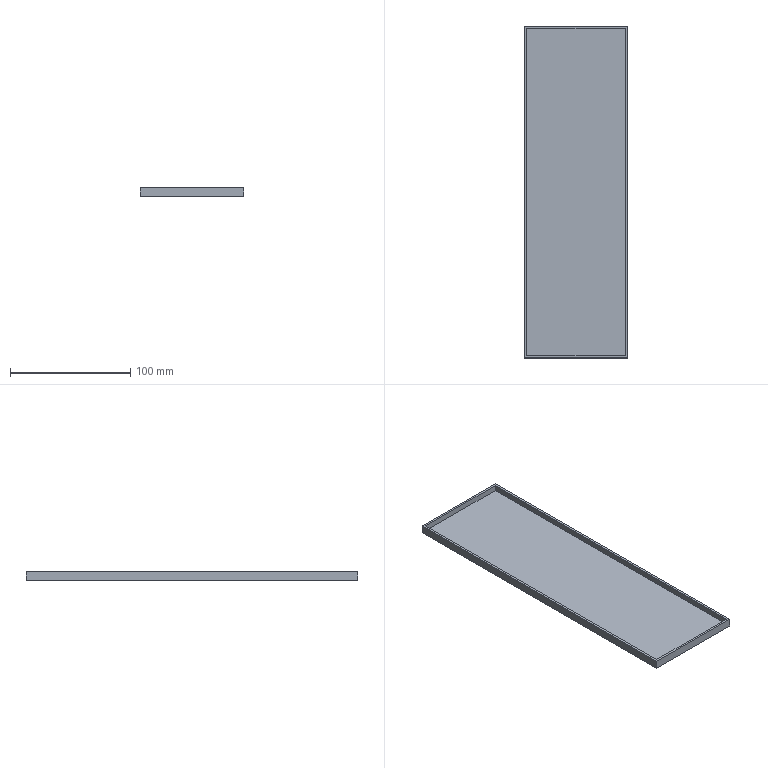Part | NX | features solid 2 | 1 solid | 11 faces | box 86 x 276 x 7 mm | volume 54632 mm3 | plane 11
STEP:
#1=CARTESIAN_POINT('',(348.,283.,-287.));
#2=VERTEX_POINT('',#1);
#3=CARTESIAN_POINT('',(348.,7.,-287.));
#4=VERTEX_POINT('',#3);
#5=CARTESIAN_POINT('',(348.,10.,-287.));
#6=DIRECTION('',(0.,-1.,0.));
#7=VECTOR('',#6,1000.);
#8=LINE('',#5,#7);
#9=EDGE_CURVE('',#2,#4,#8,.T.);
#10=ORIENTED_EDGE('',*,*,#9,.F.);
#11=CARTESIAN_POINT('',(348.,283.,-280.));
#12=VERTEX_POINT('',#11);
#13=CARTESIAN_POINT('',(348.,283.,-280.));
#14=DIRECTION('',(0.,0.,-1.));
#15=VECTOR('',#14,1000.);
#16=LINE('',#13,#15);
#17=EDGE_CURVE('',#12,#2,#16,.T.);
#18=ORIENTED_EDGE('',*,*,#17,.F.);
#19=CARTESIAN_POINT('',(348.,7.,-280.));
#20=VERTEX_POINT('',#19);
#21=CARTESIAN_POINT('',(348.,10.,-280.));
#22=DIRECTION('',(0.,-1.,0.));
#23=VECTOR('',#22,1000.);
#24=LINE('',#21,#23);
#25=EDGE_CURVE('',#12,#20,#24,.T.);
#26=ORIENTED_EDGE('',*,*,#25,.T.);
#27=CARTESIAN_POINT('',(348.,7.,-280.));
#28=DIRECTION('',(0.,0.,-1.));
#29=VECTOR('',#28,1000.);
#30=LINE('',#27,#29);
#31=EDGE_CURVE('',#20,#4,#30,.T.);
#32=ORIENTED_EDGE('',*,*,#31,.T.);
#33=EDGE_LOOP('',(#10,#18,#26,#32));
#34=FACE_BOUND('',#33,.T.);
#35=CARTESIAN_POINT('',(348.,290.,-280.));
#36=DIRECTION('',(1.,0.,0.));
#37=DIRECTION('',(0.,0.,-1.));
#38=AXIS2_PLACEMENT_3D('',#35,#36,#37);
#39=PLANE('',#38);
#40=ADVANCED_FACE('',(#34),#39,.T.);
#41=CARTESIAN_POINT('',(262.,7.,-287.));
#42=VERTEX_POINT('',#41);
#43=CARTESIAN_POINT('',(345.,7.,-287.));
#44=DIRECTION('',(-1.,0.,0.));
#45=VECTOR('',#44,1000.);
#46=LINE('',#43,#45);
#47=EDGE_CURVE('',#4,#42,#46,.T.);
#48=ORIENTED_EDGE('',*,*,#47,.F.);
#49=ORIENTED_EDGE('',*,*,#31,.F.);
#50=CARTESIAN_POINT('',(262.,7.,-280.));
#51=VERTEX_POINT('',#50);
#52=CARTESIAN_POINT('',(345.,7.,-280.));
#53=DIRECTION('',(-1.,0.,0.));
#54=VECTOR('',#53,1000.);
#55=LINE('',#52,#54);
#56=EDGE_CURVE('',#20,#51,#55,.T.);
#57=ORIENTED_EDGE('',*,*,#56,.T.);
#58=CARTESIAN_POINT('',(262.,7.,-280.));
#59=DIRECTION('',(0.,0.,-1.));
#60=VECTOR('',#59,1000.);
#61=LINE('',#58,#60);
#62=EDGE_CURVE('',#51,#42,#61,.T.);
#63=ORIENTED_EDGE('',*,*,#62,.T.);
#64=EDGE_LOOP('',(#48,#49,#57,#63));
#65=FACE_BOUND('',#64,.T.);
#66=CARTESIAN_POINT('',(345.,7.,-280.));
#67=DIRECTION('',(0.,-1.,0.));
#68=DIRECTION('',(0.,0.,-1.));
#69=AXIS2_PLACEMENT_3D('',#66,#67,#68);
#70=PLANE('',#69);
#71=ADVANCED_FACE('',(#65),#70,.T.);
#72=CARTESIAN_POINT('',(262.,283.,-287.));
#73=VERTEX_POINT('',#72);
#74=CARTESIAN_POINT('',(262.,10.,-287.));
#75=DIRECTION('',(0.,1.,0.));
#76=VECTOR('',#75,1000.);
#77=LINE('',#74,#76);
#78=EDGE_CURVE('',#42,#73,#77,.T.);
#79=ORIENTED_EDGE('',*,*,#78,.F.);
#80=ORIENTED_EDGE('',*,*,#62,.F.);
#81=CARTESIAN_POINT('',(262.,283.,-280.));
#82=VERTEX_POINT('',#81);
#83=CARTESIAN_POINT('',(262.,10.,-280.));
#84=DIRECTION('',(0.,1.,0.));
#85=VECTOR('',#84,1000.);
#86=LINE('',#83,#85);
#87=EDGE_CURVE('',#51,#82,#86,.T.);
#88=ORIENTED_EDGE('',*,*,#87,.T.);
#89=CARTESIAN_POINT('',(262.,283.,-280.));
#90=DIRECTION('',(0.,0.,-1.));
#91=VECTOR('',#90,1000.);
#92=LINE('',#89,#91);
#93=EDGE_CURVE('',#82,#73,#92,.T.);
#94=ORIENTED_EDGE('',*,*,#93,.T.);
#95=EDGE_LOOP('',(#79,#80,#88,#94));
#96=FACE_BOUND('',#95,.T.);
#97=CARTESIAN_POINT('',(262.,10.,-280.));
#98=DIRECTION('',(-1.,0.,0.));
#99=DIRECTION('',(0.,0.,1.));
#100=AXIS2_PLACEMENT_3D('',#97,#98,#99);
#101=PLANE('',#100);
#102=ADVANCED_FACE('',(#96),#101,.T.);
#103=CARTESIAN_POINT('',(345.,283.,-287.));
#104=DIRECTION('',(1.,0.,0.));
#105=VECTOR('',#104,1000.);
#106=LINE('',#103,#105);
#107=EDGE_CURVE('',#73,#2,#106,.T.);
#108=ORIENTED_EDGE('',*,*,#107,.F.);
#109=ORIENTED_EDGE('',*,*,#93,.F.);
#110=CARTESIAN_POINT('',(345.,283.,-280.));
#111=DIRECTION('',(1.,0.,0.));
#112=VECTOR('',#111,1000.);
#113=LINE('',#110,#112);
#114=EDGE_CURVE('',#82,#12,#113,.T.);
#115=ORIENTED_EDGE('',*,*,#114,.T.);
#116=ORIENTED_EDGE('',*,*,#17,.T.);
#117=EDGE_LOOP('',(#108,#109,#115,#116));
#118=FACE_BOUND('',#117,.T.);
#119=CARTESIAN_POINT('',(-690.,283.,-280.));
#120=DIRECTION('',(0.,1.,0.));
#121=DIRECTION('',(-1.,0.,0.));
#122=AXIS2_PLACEMENT_3D('',#119,#120,#121);
#123=PLANE('',#122);
#124=ADVANCED_FACE('',(#118),#123,.T.);
#125=CARTESIAN_POINT('',(264.,281.,-280.));
#126=VERTEX_POINT('',#125);
#127=CARTESIAN_POINT('',(346.,281.,-280.));
#128=VERTEX_POINT('',#127);
#129=CARTESIAN_POINT('',(345.,281.,-280.));
#130=DIRECTION('',(1.,0.,0.));
#131=VECTOR('',#130,1000.);
#132=LINE('',#129,#131);
#133=EDGE_CURVE('',#126,#128,#132,.T.);
#134=ORIENTED_EDGE('',*,*,#133,.T.);
#135=CARTESIAN_POINT('',(346.,9.,-280.));
#136=VERTEX_POINT('',#135);
#137=CARTESIAN_POINT('',(346.,10.,-280.));
#138=DIRECTION('',(0.,-1.,0.));
#139=VECTOR('',#138,1000.);
#140=LINE('',#137,#139);
#141=EDGE_CURVE('',#128,#136,#140,.T.);
#142=ORIENTED_EDGE('',*,*,#141,.T.);
#143=CARTESIAN_POINT('',(264.,9.,-280.));
#144=VERTEX_POINT('',#143);
#145=CARTESIAN_POINT('',(345.,9.,-280.));
#146=DIRECTION('',(-1.,0.,0.));
#147=VECTOR('',#146,1000.);
#148=LINE('',#145,#147);
#149=EDGE_CURVE('',#136,#144,#148,.T.);
#150=ORIENTED_EDGE('',*,*,#149,.T.);
#151=CARTESIAN_POINT('',(264.,10.,-280.));
#152=DIRECTION('',(0.,1.,0.));
#153=VECTOR('',#152,1000.);
#154=LINE('',#151,#153);
#155=EDGE_CURVE('',#144,#126,#154,.T.);
#156=ORIENTED_EDGE('',*,*,#155,.T.);
#157=EDGE_LOOP('',(#134,#142,#150,#156));
#158=FACE_BOUND('',#157,.T.);
#159=ORIENTED_EDGE('',*,*,#25,.F.);
#160=ORIENTED_EDGE('',*,*,#114,.F.);
#161=ORIENTED_EDGE('',*,*,#87,.F.);
#162=ORIENTED_EDGE('',*,*,#56,.F.);
#163=EDGE_LOOP('',(#159,#160,#161,#162));
#164=FACE_BOUND('',#163,.T.);
#165=CARTESIAN_POINT('',(345.,10.,-280.));
#166=DIRECTION('',(0.,0.,-1.));
#167=DIRECTION('',(-1.,0.,0.));
#168=AXIS2_PLACEMENT_3D('',#165,#166,#167);
#169=PLANE('',#168);
#170=ADVANCED_FACE('',(#158,#164),#169,.F.);
#171=ORIENTED_EDGE('',*,*,#9,.T.);
#172=ORIENTED_EDGE('',*,*,#47,.T.);
#173=ORIENTED_EDGE('',*,*,#78,.T.);
#174=ORIENTED_EDGE('',*,*,#107,.T.);
#175=EDGE_LOOP('',(#171,#172,#173,#174));
#176=FACE_BOUND('',#175,.T.);
#177=CARTESIAN_POINT('',(345.,10.,-287.));
#178=DIRECTION('',(0.,0.,-1.));
#179=DIRECTION('',(-1.,0.,0.));
#180=AXIS2_PLACEMENT_3D('',#177,#178,#179);
#181=PLANE('',#180);
#182=ADVANCED_FACE('',(#176),#181,.T.);
#183=CARTESIAN_POINT('',(346.,281.,-285.));
#184=VERTEX_POINT('',#183);
#185=CARTESIAN_POINT('',(346.,9.,-285.));
#186=VERTEX_POINT('',#185);
#187=CARTESIAN_POINT('',(346.,10.,-285.));
#188=DIRECTION('',(0.,-1.,0.));
#189=VECTOR('',#188,1000.);
#190=LINE('',#187,#189);
#191=EDGE_CURVE('',#184,#186,#190,.T.);
#192=ORIENTED_EDGE('',*,*,#191,.T.);
#193=CARTESIAN_POINT('',(346.,9.,-280.));
#194=DIRECTION('',(0.,0.,-1.));
#195=VECTOR('',#194,1000.);
#196=LINE('',#193,#195);
#197=EDGE_CURVE('',#136,#186,#196,.T.);
#198=ORIENTED_EDGE('',*,*,#197,.F.);
#199=ORIENTED_EDGE('',*,*,#141,.F.);
#200=CARTESIAN_POINT('',(346.,281.,-280.));
#201=DIRECTION('',(0.,0.,-1.));
#202=VECTOR('',#201,1000.);
#203=LINE('',#200,#202);
#204=EDGE_CURVE('',#128,#184,#203,.T.);
#205=ORIENTED_EDGE('',*,*,#204,.T.);
#206=EDGE_LOOP('',(#192,#198,#199,#205));
#207=FACE_BOUND('',#206,.T.);
#208=CARTESIAN_POINT('',(346.,290.,-280.));
#209=DIRECTION('',(1.,0.,0.));
#210=DIRECTION('',(0.,0.,-1.));
#211=AXIS2_PLACEMENT_3D('',#208,#209,#210);
#212=PLANE('',#211);
#213=ADVANCED_FACE('',(#207),#212,.F.);
#214=CARTESIAN_POINT('',(264.,9.,-285.));
#215=VERTEX_POINT('',#214);
#216=CARTESIAN_POINT('',(345.,9.,-285.));
#217=DIRECTION('',(-1.,0.,0.));
#218=VECTOR('',#217,1000.);
#219=LINE('',#216,#218);
#220=EDGE_CURVE('',#186,#215,#219,.T.);
#221=ORIENTED_EDGE('',*,*,#220,.T.);
#222=CARTESIAN_POINT('',(264.,9.,-280.));
#223=DIRECTION('',(0.,0.,-1.));
#224=VECTOR('',#223,1000.);
#225=LINE('',#222,#224);
#226=EDGE_CURVE('',#144,#215,#225,.T.);
#227=ORIENTED_EDGE('',*,*,#226,.F.);
#228=ORIENTED_EDGE('',*,*,#149,.F.);
#229=ORIENTED_EDGE('',*,*,#197,.T.);
#230=EDGE_LOOP('',(#221,#227,#228,#229));
#231=FACE_BOUND('',#230,.T.);
#232=CARTESIAN_POINT('',(345.,9.,-280.));
#233=DIRECTION('',(0.,-1.,0.));
#234=DIRECTION('',(0.,0.,-1.));
#235=AXIS2_PLACEMENT_3D('',#232,#233,#234);
#236=PLANE('',#235);
#237=ADVANCED_FACE('',(#231),#236,.F.);
#238=CARTESIAN_POINT('',(264.,281.,-285.));
#239=VERTEX_POINT('',#238);
#240=CARTESIAN_POINT('',(264.,10.,-285.));
#241=DIRECTION('',(0.,1.,0.));
#242=VECTOR('',#241,1000.);
#243=LINE('',#240,#242);
#244=EDGE_CURVE('',#215,#239,#243,.T.);
#245=ORIENTED_EDGE('',*,*,#244,.T.);
#246=CARTESIAN_POINT('',(264.,281.,-280.));
#247=DIRECTION('',(0.,0.,-1.));
#248=VECTOR('',#247,1000.);
#249=LINE('',#246,#248);
#250=EDGE_CURVE('',#126,#239,#249,.T.);
#251=ORIENTED_EDGE('',*,*,#250,.F.);
#252=ORIENTED_EDGE('',*,*,#155,.F.);
#253=ORIENTED_EDGE('',*,*,#226,.T.);
#254=EDGE_LOOP('',(#245,#251,#252,#253));
#255=FACE_BOUND('',#254,.T.);
#256=CARTESIAN_POINT('',(264.,10.,-280.));
#257=DIRECTION('',(-1.,0.,0.));
#258=DIRECTION('',(0.,0.,1.));
#259=AXIS2_PLACEMENT_3D('',#256,#257,#258);
#260=PLANE('',#259);
#261=ADVANCED_FACE('',(#255),#260,.F.);
#262=CARTESIAN_POINT('',(345.,281.,-285.));
#263=DIRECTION('',(1.,0.,0.));
#264=VECTOR('',#263,1000.);
#265=LINE('',#262,#264);
#266=EDGE_CURVE('',#239,#184,#265,.T.);
#267=ORIENTED_EDGE('',*,*,#266,.T.);
#268=ORIENTED_EDGE('',*,*,#204,.F.);
#269=ORIENTED_EDGE('',*,*,#133,.F.);
#270=ORIENTED_EDGE('',*,*,#250,.T.);
#271=EDGE_LOOP('',(#267,#268,#269,#270));
#272=FACE_BOUND('',#271,.T.);
#273=CARTESIAN_POINT('',(-690.,281.,-280.));
#274=DIRECTION('',(0.,1.,0.));
#275=DIRECTION('',(-1.,0.,0.));
#276=AXIS2_PLACEMENT_3D('',#273,#274,#275);
#277=PLANE('',#276);
#278=ADVANCED_FACE('',(#272),#277,.F.);
#279=ORIENTED_EDGE('',*,*,#191,.F.);
#280=ORIENTED_EDGE('',*,*,#266,.F.);
#281=ORIENTED_EDGE('',*,*,#244,.F.);
#282=ORIENTED_EDGE('',*,*,#220,.F.);
#283=EDGE_LOOP('',(#279,#280,#281,#282));
#284=FACE_BOUND('',#283,.T.);
#285=CARTESIAN_POINT('',(345.,10.,-285.));
#286=DIRECTION('',(0.,0.,-1.));
#287=DIRECTION('',(-1.,0.,0.));
#288=AXIS2_PLACEMENT_3D('',#285,#286,#287);
#289=PLANE('',#288);
#290=ADVANCED_FACE('',(#284),#289,.F.);
#291=CLOSED_SHELL('',(#40,#71,#102,#124,#170,#182,#213,#237,#261,#278,#290));
#292=MANIFOLD_SOLID_BREP('',#291);
#293=(LENGTH_UNIT()NAMED_UNIT(*)SI_UNIT(.MILLI.,.METRE.));
#294=UNCERTAINTY_MEASURE_WITH_UNIT(LENGTH_MEASURE(0.00001),#293,'','');
#295=(NAMED_UNIT(*)PLANE_ANGLE_UNIT()SI_UNIT($,.RADIAN.));
#296=(NAMED_UNIT(*)SI_UNIT($,.STERADIAN.)SOLID_ANGLE_UNIT());
#297=(GEOMETRIC_REPRESENTATION_CONTEXT(3)GLOBAL_UNCERTAINTY_ASSIGNED_CONTEXT((#294))GLOBAL_UNIT_ASSIGNED_CONTEXT((#293,#295,#296))REPRESENTATION_CONTEXT('',''));
#298=ADVANCED_BREP_SHAPE_REPRESENTATION('',(#292),#297);